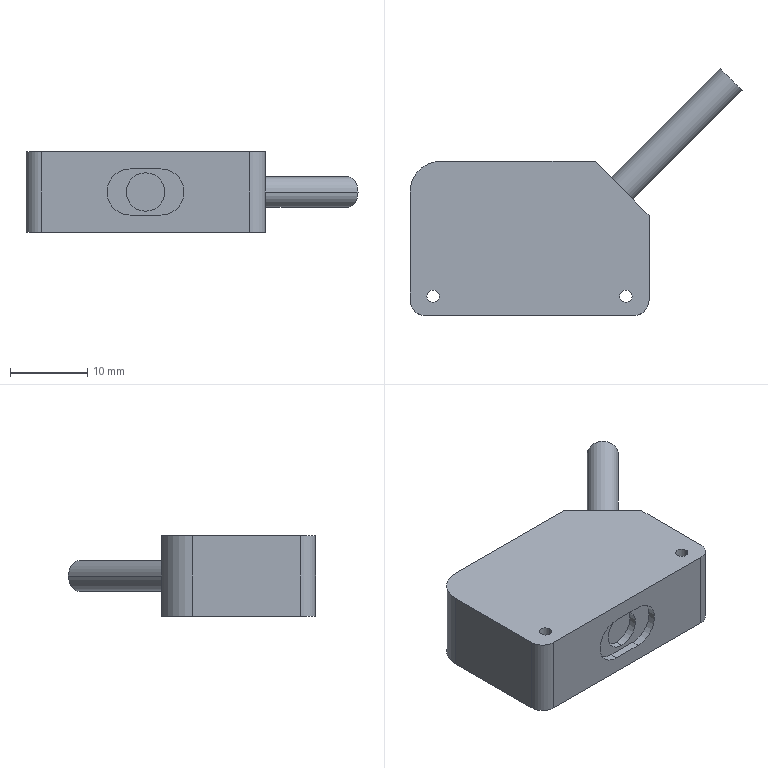Part | STEP file | E3Z-T61-L | 1 solid | 25 faces | box 43.056 x 32.056 x 10.4 mm | volume 6277 mm3 | cylinder 13 | plane 12 | commonest cylinder face diameters 1.6 x4 4 x4 5 x2 6 x2 8 x1